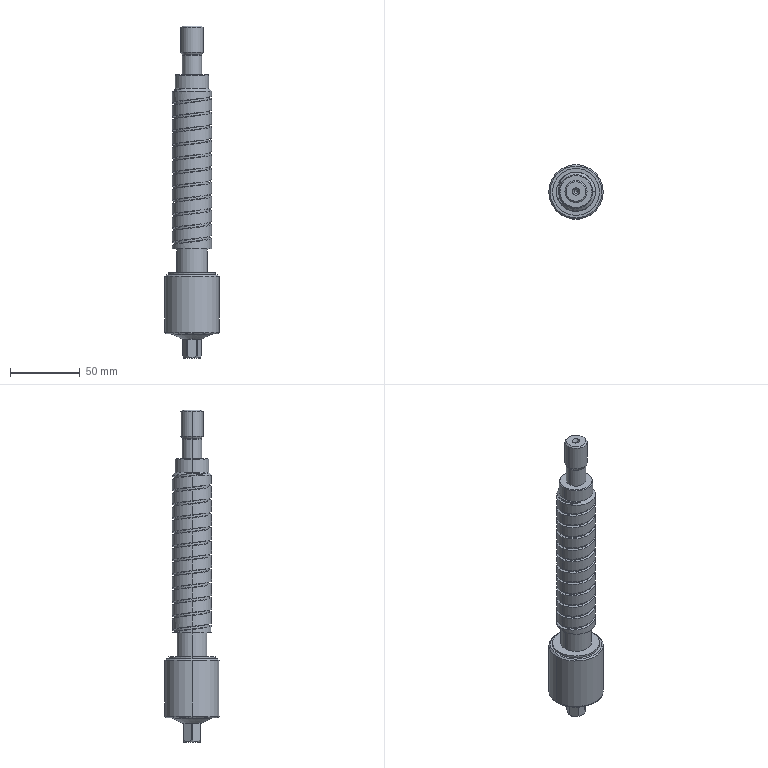Part | SolidWorks | features ICE 3, BaseBody 1, Chamfer 1, Helix 1, MoveCopyBody 1, Split 1, SweepCut 1 | 3 solids | 102 faces | box 39 x 39 x 238 mm | volume 139894 mm3 | cylinder 48 | cone 24 | plane 21 | spline 9 | commonest cylinder face diameters 28 x25 13.5 x7 2.5 x4 13.9 x2 16 x2 22 x2